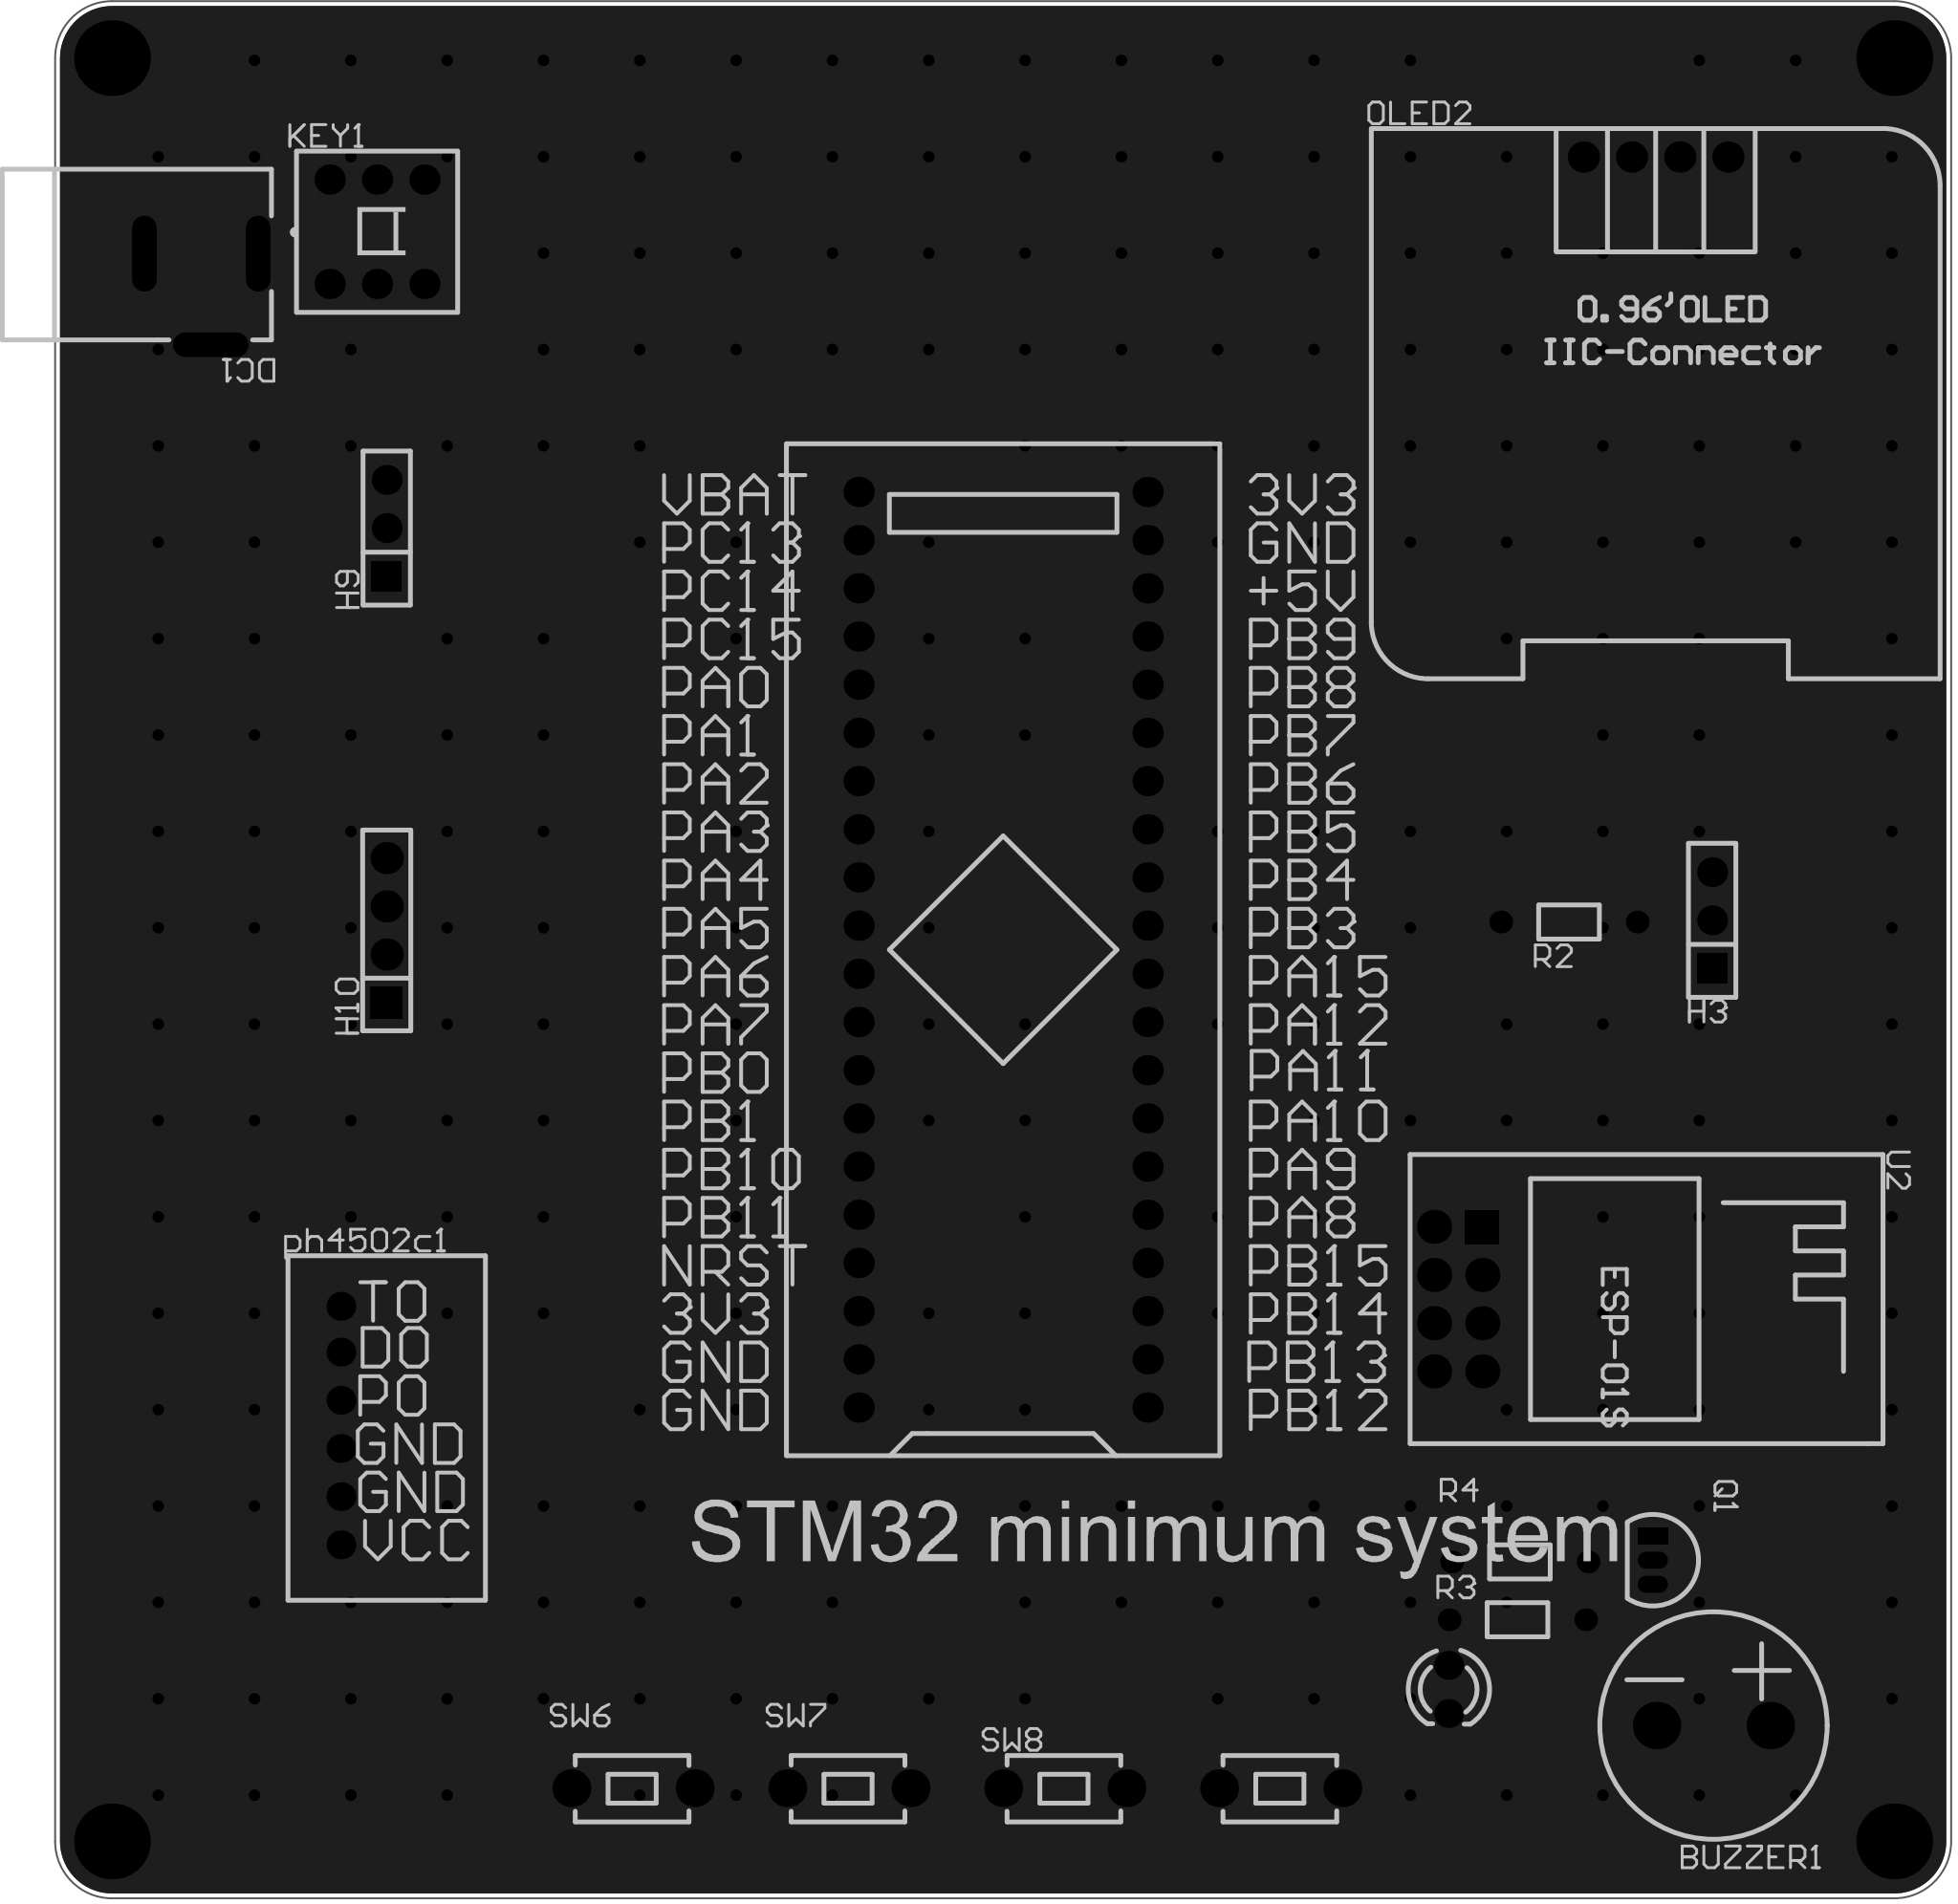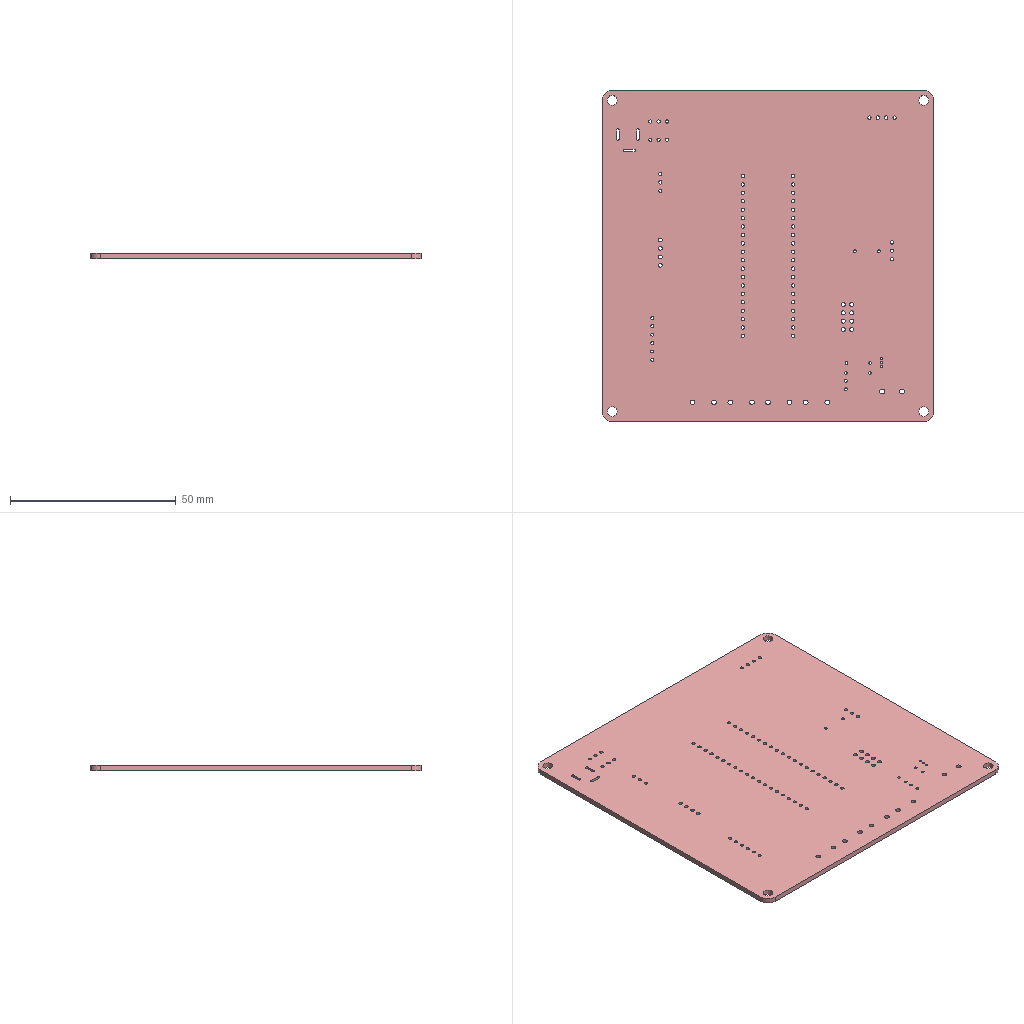Circuit board layout | Altium Designer | box 100 x 100 x 1.6 mm
Layer stack:
# Altium Designer layer stack of  (unit mm; dielectric type: 0 none, 1 core, 2 prepreg, 3 surface material)
index,name,kind,layer,copper_thickness_mm,dielectric_type,dielectric_thickness_mm,dielectric_material,dielectric_constant
0,Top Paste Mask Layer,other,,,,,,
1,Top Silkscreen Layer,other,,,,,,
2,Top Solder Mask Layer,dielectric,,,3,0.01,,3.3
3,Top Layer,copper,Top Layer,0.035,,,,
4,Dielectric1,dielectric,,,3,1.51,FR4,4.5
5,Bottom Layer,copper,Bottom Layer,0.035,,,,
6,Bottom Solder Mask Layer,dielectric,,,3,0.01,,3.3
7,Bottom Silkscreen Layer,other,,,,,,
8,Bottom Paste Mask Layer,other,,,,,,
# drill layer pairs: low layer,high layer
drill_pair,Top Layer,Bottom Layer
Part placement:
Designator,Comment,Layer,Footprint,Center-X(mm),Center-Y(mm),Rotation
U1,STM32F103C8T6-Card,TopLayer,CONN-TH_L53.3-W22.9_STM32F103C8T6-CARD,141.351,130.937,90
BUZZER1,buzzer,TopLayer,BUZ-TH_BD12.0-P6.00-D0.9-RD,178.816,90.043,0
DC1,,TopLayer,DC-2.0,99.06,165.227,180
H3,,TopLayer,HDR-TH_3P-P2.54-V-F,178.745,132.487,90
H9,,TopLayer,HDR-TH_3P-P2.54-V-F,108.839,153.162,90
H10,,TopLayer,HDR-TH_4P-P2.54-V-F,108.839,131.955,90
LED2,,TopLayer,LED_TH-3mm,164.846,91.948,270
KEY1,Non-self-locking switch 8.5×8.5 silent,TopLayer,SW-TH_6P-L8.5-W8.5-P2.54,108.331,168.783,0
OLED2,,TopLayer,0.96OLED_4P,175.768,172.72,0
ph4502c1,,TopLayer,PH4502C,106.426,105.855,0
R2,100,TopLayer,Res_1/8W,171.196,132.398,180
R3,10kΩ,TopLayer,Res_1/8W,168.478,95.621,0
Q1,,TopLayer,S8050_TO_92,175.616,98.759,270
R4,1kΩ,TopLayer,Res_1/8W,168.605,98.669,0
SW6,,TopLayer,Key_TH_3.5x6x4.3,121.831,86.741,0
SW7,,TopLayer,Key_TH_3.5x6x4.3,133.219,86.741,0
SW9,,TopLayer,Key_TH_3.5x6x4.3,155.994,86.741,0
SW8,,TopLayer,Key_TH_3.5x6x4.3,144.607,86.741,0
U2,ESP-01S,TopLayer,WIFIM-TH_ESP-01S,165.354,112.522,270
Pad and via stacks:
# Altium Designer via and pad stacks of  (unit mm). Each distinct definition once, with the count of objects using it.
# via: kind,start_layer,end_layer,hole_mm,diameter_mm,mode(0 simple;1 top-mid-bottom;2 full stack),diameter_per_layer,count,example_net
# pad: kind,layer,hole_mm,hole_type(0 round;1 square;2 slot),plating,top_size,top_shape(1 round;2 rect;3 octagon;9 rounded rect),mid_size,bottom_size,mode,footprint,size_per_layer,count,example
pad,Multi-Layer,3,0,plated,4x4,1,4x4,4x4,0,,,4,1
pad,Multi-Layer,1,0,plated,1.6x1.6,1,1.6x1.6,1.6x1.6,0,CONN-TH_L53.3-W22.9_STM32F103C8T6-CARD,,40,U1.1
pad,Multi-Layer,1.5,0,plated,2.5x2.5,1,2.5x2.5,2.5x2.5,0,BUZ-TH_BD12.0-P6.00-D0.9-RD,,2,BUZZER1.1
pad,Multi-Layer,0.8001,2,plated,4x1.3,1,4x1.3,4x1.3,0,DC-2.0,,3,DC1.2
pad,Multi-Layer,1.02,0,plated,1.575x1.575,1,1.575x1.575,1.575x1.575,0,HDR-TH_3P-P2.54-V-F,,4,H3.3
pad,Multi-Layer,1.02,0,plated,1.575x1.575,2,1.575x1.575,1.575x1.575,0,HDR-TH_3P-P2.54-V-F,,2,H3.1
pad,Multi-Layer,1.1,0,plated,1.7x1.7,2,1.7x1.7,1.7x1.7,0,HDR-TH_4P-P2.54-V-F,,1,H10.1
pad,Multi-Layer,1.1,0,plated,1.7x1.7,1,1.7x1.7,1.7x1.7,0,HDR-TH_4P-P2.54-V-F,,3,H10.2
pad,Multi-Layer,0.9144,0,plated,1.524x1.524,1,1.524x1.524,1.524x1.524,0,LED_TH-3mm,,2,LED2.1
pad,Multi-Layer,1,0,plated,1.6x1.6,1,1.6x1.6,1.6x1.6,0,SW-TH_6P-L8.5-W8.5-P2.54,,6,KEY1.4
pad,Multi-Layer,1,0,plated,1.65x1.65,1,1.65x1.65,1.65x1.65,0,0.96OLED_4P,,4,OLED2.4
pad,Multi-Layer,0.9144,0,plated,1.524x1.524,1,1.524x1.524,1.524x1.524,0,PH4502C,,6,ph4502c1.1
pad,Multi-Layer,0.8001,0,plated,1.199x1.199,1,1.199x1.199,1.199x1.199,0,Res_1/8W,,6,R2.1
pad,Multi-Layer,0.701,0,plated,0.8992x1.6,2,0.8992x1.6,0.8992x1.6,0,S8050_TO_92,,1,Q1.1
pad,Multi-Layer,0.701,0,plated,0.8992x1.6,1,0.8992x1.6,0.8992x1.6,0,S8050_TO_92,,2,Q1.2
pad,Multi-Layer,1.399,0,plated,1.999x1.999,1,1.999x1.999,1.999x1.999,0,Key_TH_3.5x6x4.3,,8,SW6.A
pad,Multi-Layer,1.2,0,plated,1.8x1.8,2,1.8x1.8,1.8x1.8,0,WIFIM-TH_ESP-01S,,1,U2.1
pad,Multi-Layer,1.2,0,plated,1.8x1.8,1,1.8x1.8,1.8x1.8,0,WIFIM-TH_ESP-01S,,7,U2.2
via,Top Layer,Bottom Layer,0.3048,0.61,0,,263,GND
Copper pours:
name,layer,net,type(0 solid;1 hatched;2 none)
Bottom Layer-GND,Bottom Layer,GND,0
Top Layer-GND,Top Layer,GND,0
Design rules, without the lines most boards share:
# Altium Designer design rules of  (exported by Altium Designer, unit mm)
# columns: name | kind | enabled | priority | scope1 | scope2 | descriptor | typed fields (field=value)
Copper_copperRegion_copperThickness1oz | 0 | disabled | 4 | All | All | Clearance Constraint (Gap=5.984mil) (Disabled)(All),(All) | gap=0.152
Copper_copperRegion_copperThickness1oz_1 | 63 | disabled | 4 | All | All | Board Clearance Constraint (Gap=0mil) (Disabled)(All) |
Copper_copperRegion_Copper_copperRegion | 0 | disabled | 5 | All | All | Clearance Constraint (Gap=5.984mil) (Disabled)(All),(All) | gap=0.152
Copper_copperRegion_Copper_copperRegion_1 | 63 | disabled | 5 | All | All | Board Clearance Constraint (Gap=0mil) (Disabled)(All) |
copperThickness1oz | 0 | enabled | 6 | All | All | Clearance Constraint (Gap=5.984mil) (All),(All) | gap=0.152
copperThickness1oz_1 | 63 | enabled | 6 | All | All | Board Clearance Constraint (Gap=0mil) (All) |
copperRegion_copperThickness1oz | 20 | disabled | 1 | All | All | Polygon Connect Rule(Relief Connect )(Conductor Width=10mil) (Relief Angle=90 Angle) (Entries=4) (Air Gap Width=10mil) (Disabled)(All),(All) | connect_style(0=relief,1=direct,2=none)=0 relief_conductor_width=0.254 relief_entries=4
copperRegion_Copper_copperRegion | 20 | disabled | 2 | All | All | Polygon Connect Rule(Relief Connect )(Conductor Width=10mil) (Relief Angle=90 Angle) (Entries=4) (Air Gap Width=10mil) (Disabled)(All),(All) | connect_style(0=relief,1=direct,2=none)=0 relief_conductor_width=0.254 relief_entries=4
copperRegion | 20 | enabled | 3 | All | All | Polygon Connect Rule(Relief Connect )(Conductor Width=10mil) (Relief Angle=90 Angle) (Entries=4) (Air Gap Width=10mil) (All),(All) | connect_style(0=relief,1=direct,2=none)=0 relief_conductor_width=0.254 relief_entries=4